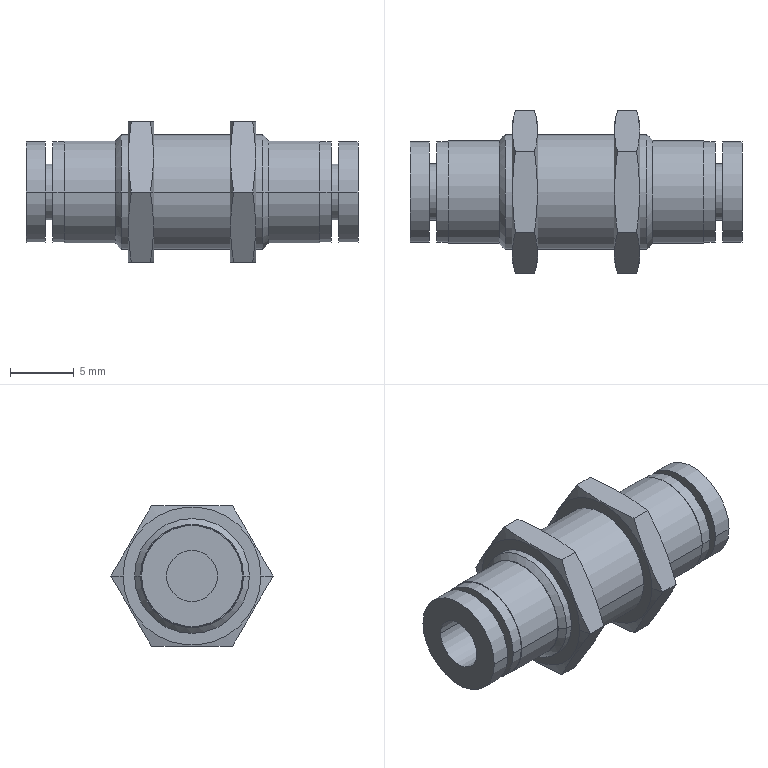Part | NX | features BREP 3 | 3 solids | 74 faces | box 26 x 12.702 x 11 mm | volume 1290 mm3 | plane 28 | cylinder 26 | cone 20 | commonest cylinder face diameters 7.9 x8 4 x4 4.4 x4 8 x4 8.188 x4 9 x2